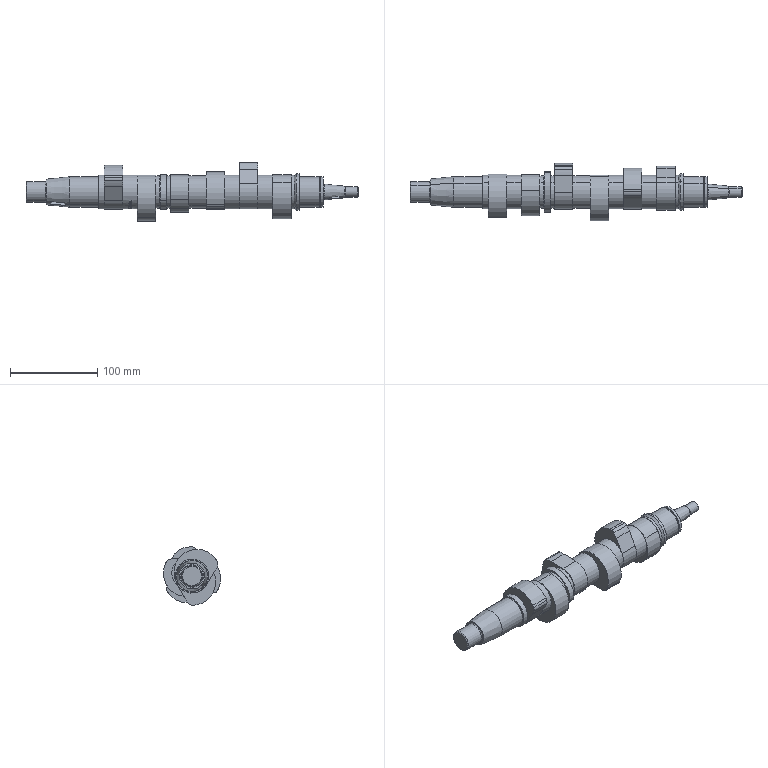Part | SolidWorks | features BaseBody 1 | 1 solid | 236 faces | box 380 x 65.688 x 67 mm | volume 451295 mm3 | cylinder 79 | plane 67 | spline 62 | torus 18 | cone 10 | commonest cylinder face diameters 38.5 x15 39 x9 53 x8 10 x7 35 x6 37 x6